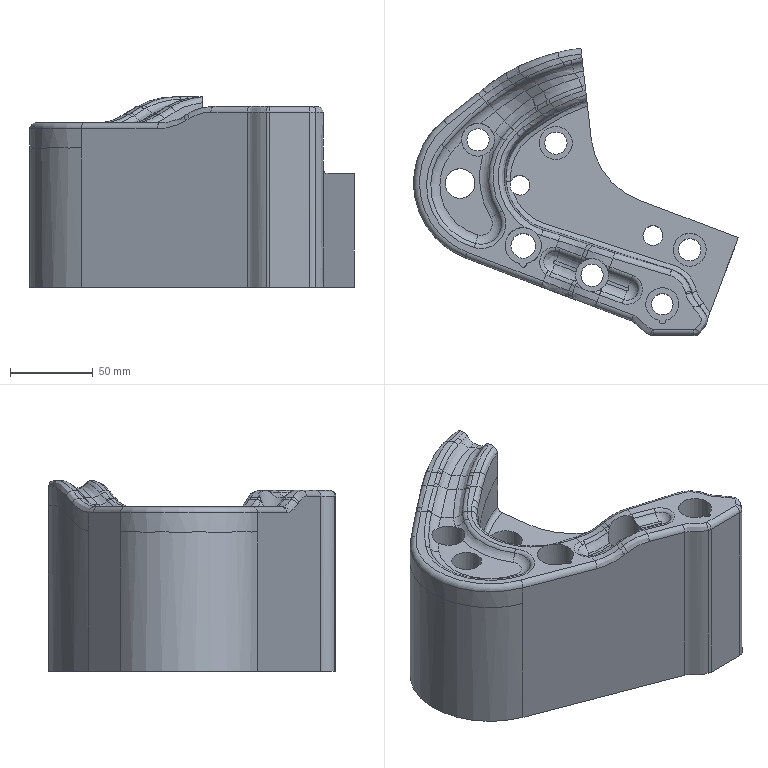Part | NX | features 23 2 | 1 solid | 168 faces | box 196.558 x 173.853 x 115.4 mm | volume 1415300 mm3 | spline 64 | cylinder 50 | plane 27 | torus 27 | commonest cylinder face diameters 7 x6 13 x5 20 x5 6 x4 13.5 x4 4 x2